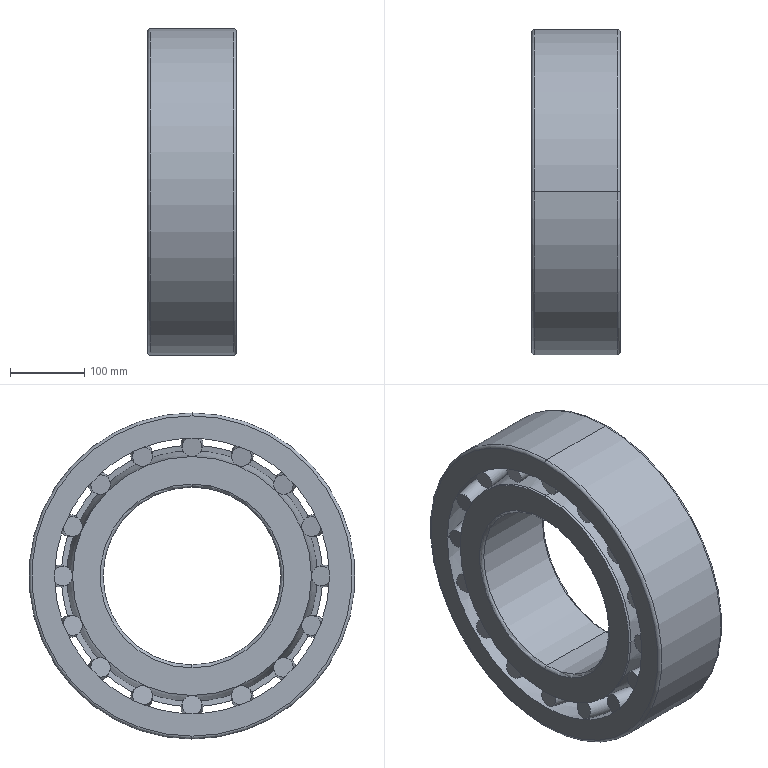Part | SolidWorks | features Revolution 3, CirPattern 1, MirrorPattern 1 | 1 solid | 188 faces | box 120 x 440 x 440 mm | volume 10049634 mm3 | torus 80 | plane 68 | cone 32 | cylinder 6 | sphere 2 | commonest cylinder face diameters 240 x2 352.5 x2 440 x2